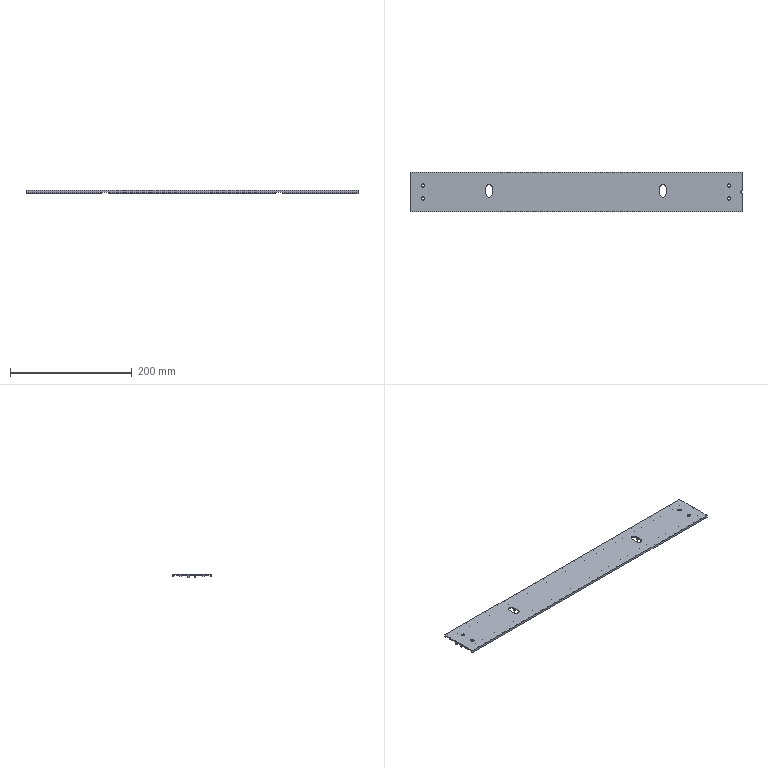Part | NX | features solid 2 | 1 solid | 60 faces | box 544.5 x 64 x 6 mm | volume 78668 mm3 | plane 47 | cylinder 13 | commonest cylinder face diameters 5.437 x8 10.5 x4 3.742 x1